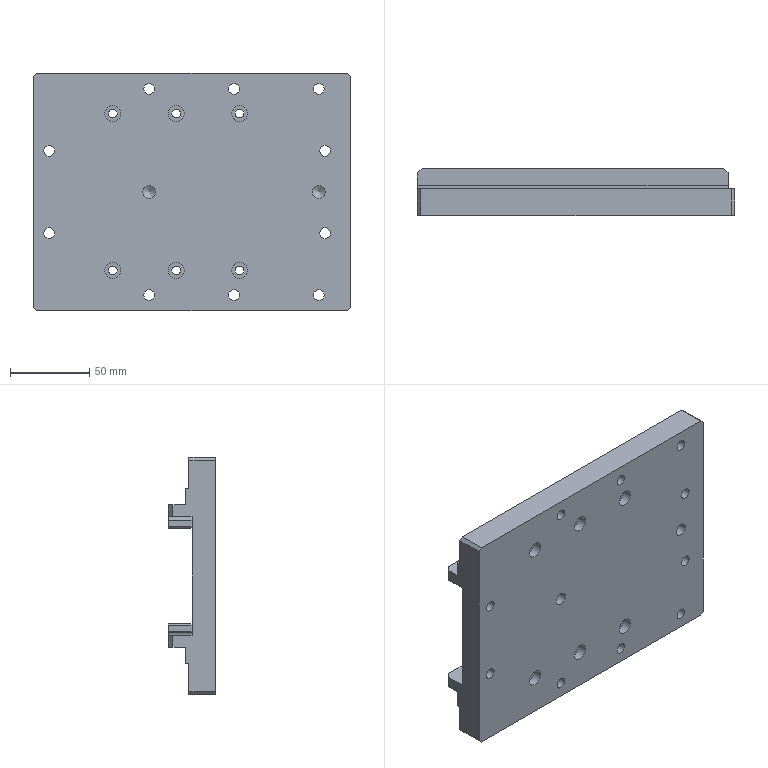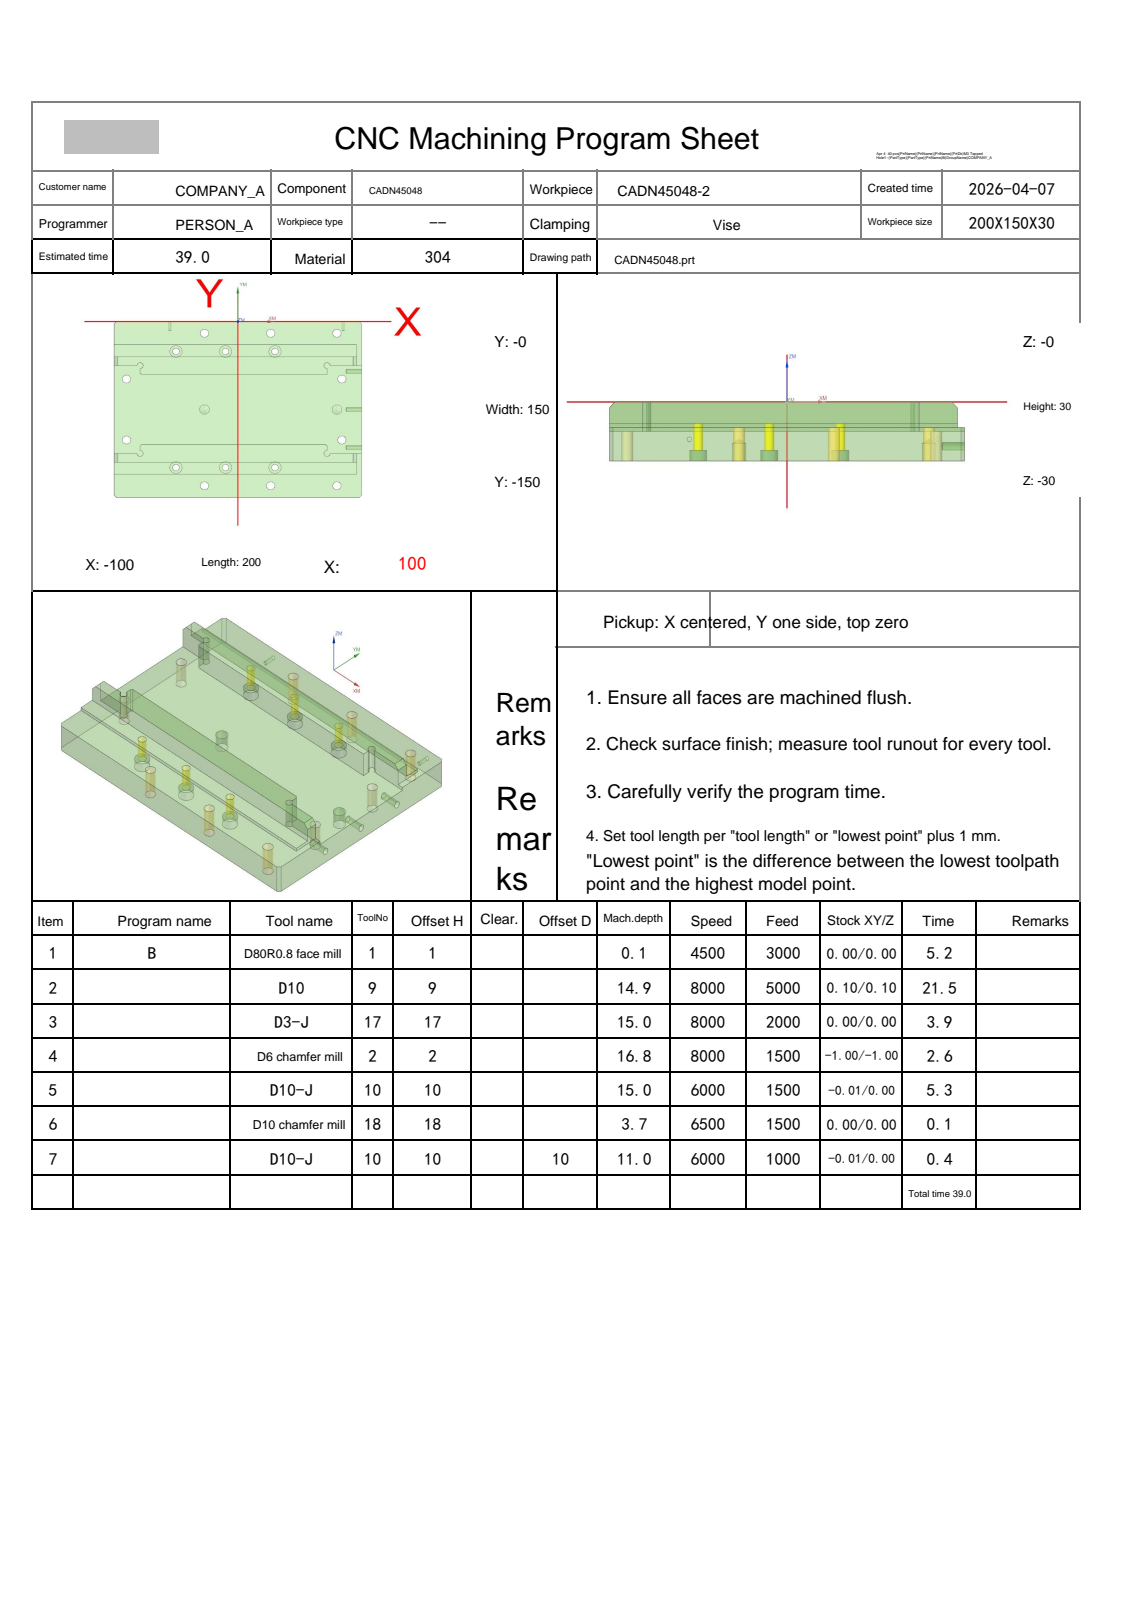NC program | NX | posted by the shop | part box 200 x 30 x 150 mm
Lines 6574 to 7628 of 19220:
N3 T17 M06
(D3-J  D=3. R=0. H=17 ce=0.00 di=0.00)
G00 G90 G54 X77.275 Y-39.301 M03 S8000
G43 H17 Z20.
M08
Z.15
G01 X77.274 Y-39.297 Z.104 F2000.
X77.272 Y-39.286 Z.063
X77.267 Y-39.27 Z.027
X77.26 Y-39.248 Z-.006
X77.251 Y-39.223 Z-.034
X77.239 Y-39.195 Z-.059
X77.224 Y-39.166 Z-.081
X77.206 Y-39.135 Z-.099
X77.185 Y-39.106 Z-.114
X77.16 Y-39.078 Z-.126
X77.131 Y-39.053 Z-.135
X77.099 Y-39.031 Z-.142
X77.062 Y-39.015 Z-.147
X77.021 Y-39.004 Z-.149
X76.975 Y-39. Z-.15
X74.5
G02 X73. Y-37.5 I0.0 J1.5
G03 X72. Y-36.5 I-1. J0.0
X71. Y-37.5 I0.0 J-1.
X72. Y-38.5 I1. J0.0
G02 X73.5 Y-40. I0.0 J-1.5
G01 Y-42.475
X73.514 Y-42.504
X73.555 Y-42.508 Z-.152
X73.619 Y-42.491 Z-.154
X73.705 Y-42.453 Z-.157
X73.809 Y-42.398 Z-.16
X73.929 Y-42.326 Z-.164
X74.202 Y-42.141 Z-.174
X74.38 Y-42.011 Z-.18
X74.671 Y-41.786 Z-.191
X75.106 Y-41.414 Z-.208
X75.528 Y-41.013 Z-.225
X75.93 Y-40.592 Z-.242
X76.299 Y-40.16 Z-.259
X76.522 Y-39.872 Z-.27
X76.65 Y-39.695 Z-.276
X76.832 Y-39.424 Z-.286
X76.902 Y-39.306 Z-.29
X76.957 Y-39.203 Z-.293
X76.993 Y-39.118 Z-.296
X77.009 Y-39.054 Z-.298
X77.004 Y-39.014 Z-.3
X76.975 Y-39.
X74.5
G02 X73. Y-37.5 I0.0 J1.5
G03 X72. Y-36.5 I-1. J0.0
X71. Y-37.5 I0.0 J-1.
X72. Y-38.5 I1. J0.0
G02 X73.5 Y-40. I0.0 J-1.5
G01 Y-42.475
X73.514 Y-42.504
X73.555 Y-42.508 Z-.302
X73.619 Y-42.491 Z-.304
X73.705 Y-42.453 Z-.307
X73.809 Y-42.398 Z-.31
X73.929 Y-42.326 Z-.314
X74.202 Y-42.141 Z-.324
X74.38 Y-42.011 Z-.33
X74.671 Y-41.786 Z-.341
X75.106 Y-41.414 Z-.358
X75.528 Y-41.013 Z-.375
X75.93 Y-40.592 Z-.392
X76.299 Y-40.16 Z-.409
X76.522 Y-39.872 Z-.42
X76.65 Y-39.695 Z-.426
X76.832 Y-39.424 Z-.436
X76.902 Y-39.306 Z-.44
X76.957 Y-39.203 Z-.443
X76.993 Y-39.118 Z-.446
X77.009 Y-39.054 Z-.448
X77.004 Y-39.014 Z-.45
X76.975 Y-39.
X74.5
G02 X73. Y-37.5 I0.0 J1.5
G03 X72. Y-36.5 I-1. J0.0
X71. Y-37.5 I0.0 J-1.
X72. Y-38.5 I1. J0.0
G02 X73.5 Y-40. I0.0 J-1.5
G01 Y-42.475
X73.514 Y-42.504
X73.555 Y-42.508 Z-.452
X73.619 Y-42.491 Z-.454
X73.705 Y-42.453 Z-.457
X73.809 Y-42.398 Z-.46
X73.929 Y-42.326 Z-.464
X74.202 Y-42.141 Z-.474
X74.38 Y-42.011 Z-.48
X74.671 Y-41.786 Z-.491
X75.106 Y-41.414 Z-.508
X75.528 Y-41.013 Z-.525
X75.93 Y-40.592 Z-.542
X76.299 Y-40.16 Z-.559
X76.522 Y-39.872 Z-.57
X76.65 Y-39.695 Z-.576
X76.832 Y-39.424 Z-.586
X76.902 Y-39.306 Z-.59
X76.957 Y-39.203 Z-.593
X76.993 Y-39.118 Z-.596
X77.009 Y-39.054 Z-.598
X77.004 Y-39.014 Z-.6
X76.975 Y-39.
X74.5
G02 X73. Y-37.5 I0.0 J1.5
G03 X72. Y-36.5 I-1. J0.0
X71. Y-37.5 I0.0 J-1.
X72. Y-38.5 I1. J0.0
G02 X73.5 Y-40. I0.0 J-1.5
G01 Y-42.475
X73.514 Y-42.504
X73.555 Y-42.508 Z-.602
X73.619 Y-42.491 Z-.604
X73.705 Y-42.453 Z-.607
X73.809 Y-42.398 Z-.61
X73.929 Y-42.326 Z-.614
X74.202 Y-42.141 Z-.624
X74.38 Y-42.011 Z-.63
X74.671 Y-41.786 Z-.641
X75.106 Y-41.414 Z-.658
X75.528 Y-41.013 Z-.675
X75.93 Y-40.592 Z-.692
X76.299 Y-40.16 Z-.709
X76.522 Y-39.872 Z-.72
X76.65 Y-39.695 Z-.726
X76.832 Y-39.424 Z-.736
X76.902 Y-39.306 Z-.74
X76.957 Y-39.203 Z-.743
X76.993 Y-39.118 Z-.746
X77.009 Y-39.054 Z-.748
X77.004 Y-39.014 Z-.75
X76.975 Y-39.
X74.5
G02 X73. Y-37.5 I0.0 J1.5
G03 X72. Y-36.5 I-1. J0.0
X71. Y-37.5 I0.0 J-1.
X72. Y-38.5 I1. J0.0
G02 X73.5 Y-40. I0.0 J-1.5
G01 Y-42.475
X73.514 Y-42.504
X73.555 Y-42.508 Z-.752
X73.619 Y-42.491 Z-.754
X73.705 Y-42.453 Z-.757
X73.809 Y-42.398 Z-.76
X73.929 Y-42.326 Z-.764
X74.202 Y-42.141 Z-.774
X74.38 Y-42.011 Z-.78
X74.671 Y-41.786 Z-.791
X75.106 Y-41.414 Z-.808
X75.528 Y-41.013 Z-.825
X75.93 Y-40.592 Z-.842
X76.299 Y-40.16 Z-.859
X76.522 Y-39.872 Z-.87
X76.65 Y-39.695 Z-.876
X76.832 Y-39.424 Z-.886
X76.902 Y-39.306 Z-.89
X76.957 Y-39.203 Z-.893
X76.993 Y-39.118 Z-.896
X77.009 Y-39.054 Z-.898
X77.004 Y-39.014 Z-.9
X76.975 Y-39.
X74.5
G02 X73. Y-37.5 I0.0 J1.5
G03 X72. Y-36.5 I-1. J0.0
X71. Y-37.5 I0.0 J-1.
X72. Y-38.5 I1. J0.0
G02 X73.5 Y-40. I0.0 J-1.5
G01 Y-42.475
X73.514 Y-42.504
X73.555 Y-42.508 Z-.902
X73.619 Y-42.491 Z-.904
X73.705 Y-42.453 Z-.907
X73.809 Y-42.398 Z-.91
X73.929 Y-42.326 Z-.914
X74.202 Y-42.141 Z-.924
X74.38 Y-42.011 Z-.93
X74.671 Y-41.786 Z-.941
X75.106 Y-41.414 Z-.958
X75.528 Y-41.013 Z-.975
X75.93 Y-40.592 Z-.992
X76.299 Y-40.16 Z-1.009
X76.522 Y-39.872 Z-1.02
X76.65 Y-39.695 Z-1.026
X76.832 Y-39.424 Z-1.036
X76.902 Y-39.306 Z-1.04
X76.957 Y-39.203 Z-1.043
X76.993 Y-39.118 Z-1.046
X77.009 Y-39.054 Z-1.048
X77.004 Y-39.014 Z-1.05
X76.975 Y-39.
X74.5
G02 X73. Y-37.5 I0.0 J1.5
G03 X72. Y-36.5 I-1. J0.0
X71. Y-37.5 I0.0 J-1.
X72. Y-38.5 I1. J0.0
G02 X73.5 Y-40. I0.0 J-1.5
G01 Y-42.475
X73.514 Y-42.504
X73.555 Y-42.508 Z-1.052
X73.619 Y-42.491 Z-1.054
X73.705 Y-42.453 Z-1.057
X73.809 Y-42.398 Z-1.06
X73.929 Y-42.326 Z-1.064
X74.202 Y-42.141 Z-1.074
X74.38 Y-42.011 Z-1.08
X74.671 Y-41.786 Z-1.091
X75.106 Y-41.414 Z-1.108
X75.528 Y-41.013 Z-1.125
X75.93 Y-40.592 Z-1.142
X76.299 Y-40.16 Z-1.159
X76.522 Y-39.872 Z-1.17
X76.65 Y-39.695 Z-1.176
X76.832 Y-39.424 Z-1.186
X76.902 Y-39.306 Z-1.19
X76.957 Y-39.203 Z-1.193
X76.993 Y-39.118 Z-1.196
X77.009 Y-39.054 Z-1.198
X77.004 Y-39.014 Z-1.2
X76.975 Y-39.
X74.5
G02 X73. Y-37.5 I0.0 J1.5
G03 X72. Y-36.5 I-1. J0.0
X71. Y-37.5 I0.0 J-1.
X72. Y-38.5 I1. J0.0
G02 X73.5 Y-40. I0.0 J-1.5
G01 Y-42.475
X73.514 Y-42.504
X73.555 Y-42.508 Z-1.202
X73.619 Y-42.491 Z-1.204
X73.705 Y-42.453 Z-1.207
X73.809 Y-42.398 Z-1.21
X73.929 Y-42.326 Z-1.214
X74.202 Y-42.141 Z-1.224
X74.38 Y-42.011 Z-1.23
X74.671 Y-41.786 Z-1.241
X75.106 Y-41.414 Z-1.258
X75.528 Y-41.013 Z-1.275
X75.93 Y-40.592 Z-1.292
X76.299 Y-40.16 Z-1.309
X76.522 Y-39.872 Z-1.32
X76.65 Y-39.695 Z-1.326
X76.832 Y-39.424 Z-1.336
X76.902 Y-39.306 Z-1.34
X76.957 Y-39.203 Z-1.343
X76.993 Y-39.118 Z-1.346
X77.009 Y-39.054 Z-1.348
X77.004 Y-39.014 Z-1.35
X76.975 Y-39.
X74.5
G02 X73. Y-37.5 I0.0 J1.5
G03 X72. Y-36.5 I-1. J0.0
X71. Y-37.5 I0.0 J-1.
X72. Y-38.5 I1. J0.0
G02 X73.5 Y-40. I0.0 J-1.5
G01 Y-42.475
X73.514 Y-42.504
X73.555 Y-42.508 Z-1.352
X73.619 Y-42.491 Z-1.354
X73.705 Y-42.453 Z-1.357
X73.809 Y-42.398 Z-1.36
X73.929 Y-42.326 Z-1.364
X74.202 Y-42.141 Z-1.374
X74.38 Y-42.011 Z-1.38
X74.671 Y-41.786 Z-1.391
X75.106 Y-41.414 Z-1.408
X75.528 Y-41.013 Z-1.425
X75.93 Y-40.592 Z-1.442
X76.299 Y-40.16 Z-1.459
X76.522 Y-39.872 Z-1.47
X76.65 Y-39.695 Z-1.476
X76.832 Y-39.424 Z-1.486
X76.902 Y-39.306 Z-1.49
X76.957 Y-39.203 Z-1.493
X76.993 Y-39.118 Z-1.496
X77.009 Y-39.054 Z-1.498
X77.004 Y-39.014 Z-1.5
X76.975 Y-39.
X74.5
G02 X73. Y-37.5 I0.0 J1.5
G03 X72. Y-36.5 I-1. J0.0
X71. Y-37.5 I0.0 J-1.
X72. Y-38.5 I1. J0.0
G02 X73.5 Y-40. I0.0 J-1.5
G01 Y-42.475
X73.514 Y-42.504
X73.555 Y-42.508 Z-1.502
X73.619 Y-42.491 Z-1.504
X73.705 Y-42.453 Z-1.507
X73.809 Y-42.398 Z-1.51
X73.929 Y-42.326 Z-1.514
X74.202 Y-42.141 Z-1.524
X74.38 Y-42.011 Z-1.53
X74.671 Y-41.786 Z-1.541
X75.106 Y-41.414 Z-1.558
X75.528 Y-41.013 Z-1.575
X75.93 Y-40.592 Z-1.592
X76.299 Y-40.16 Z-1.609
X76.522 Y-39.872 Z-1.62
X76.65 Y-39.695 Z-1.626
X76.832 Y-39.424 Z-1.636
X76.902 Y-39.306 Z-1.64
X76.957 Y-39.203 Z-1.643
X76.993 Y-39.118 Z-1.646
X77.009 Y-39.054 Z-1.648
X77.004 Y-39.014 Z-1.65
X76.975 Y-39.
X74.5
G02 X73. Y-37.5 I0.0 J1.5
G03 X72. Y-36.5 I-1. J0.0
X71. Y-37.5 I0.0 J-1.
X72. Y-38.5 I1. J0.0
G02 X73.5 Y-40. I0.0 J-1.5
G01 Y-42.475
X73.514 Y-42.504
X73.555 Y-42.508 Z-1.652
X73.619 Y-42.491 Z-1.654
X73.705 Y-42.453 Z-1.657
X73.809 Y-42.398 Z-1.66
X73.929 Y-42.326 Z-1.664
X74.202 Y-42.141 Z-1.674
X74.38 Y-42.011 Z-1.68
X74.671 Y-41.786 Z-1.691
X75.106 Y-41.414 Z-1.708
X75.528 Y-41.013 Z-1.725
X75.93 Y-40.592 Z-1.742
X76.299 Y-40.16 Z-1.759
X76.522 Y-39.872 Z-1.77
X76.65 Y-39.695 Z-1.776
X76.832 Y-39.424 Z-1.786
X76.902 Y-39.306 Z-1.79
X76.957 Y-39.203 Z-1.793
X76.993 Y-39.118 Z-1.796
X77.009 Y-39.054 Z-1.798
X77.004 Y-39.014 Z-1.8
X76.975 Y-39.
X74.5
G02 X73. Y-37.5 I0.0 J1.5
G03 X72. Y-36.5 I-1. J0.0
X71. Y-37.5 I0.0 J-1.
X72. Y-38.5 I1. J0.0
G02 X73.5 Y-40. I0.0 J-1.5
G01 Y-42.475
X73.514 Y-42.504
X73.555 Y-42.508 Z-1.802
X73.619 Y-42.491 Z-1.804
X73.705 Y-42.453 Z-1.807
X73.809 Y-42.398 Z-1.81
X73.929 Y-42.326 Z-1.814
X74.202 Y-42.141 Z-1.824
X74.38 Y-42.011 Z-1.83
X74.671 Y-41.786 Z-1.841
X75.106 Y-41.414 Z-1.858
X75.528 Y-41.013 Z-1.875
X75.93 Y-40.592 Z-1.892
X76.299 Y-40.16 Z-1.909
X76.522 Y-39.872 Z-1.92
X76.65 Y-39.695 Z-1.926
X76.832 Y-39.424 Z-1.936
X76.902 Y-39.306 Z-1.94
X76.957 Y-39.203 Z-1.943
X76.993 Y-39.118 Z-1.946
X77.009 Y-39.054 Z-1.948
X77.004 Y-39.014 Z-1.95
X76.975 Y-39.
X74.5
G02 X73. Y-37.5 I0.0 J1.5
G03 X72. Y-36.5 I-1. J0.0
X71. Y-37.5 I0.0 J-1.
X72. Y-38.5 I1. J0.0
G02 X73.5 Y-40. I0.0 J-1.5
G01 Y-42.475
X73.514 Y-42.504
X73.555 Y-42.508 Z-1.952
X73.619 Y-42.491 Z-1.954
X73.705 Y-42.453 Z-1.957
X73.809 Y-42.398 Z-1.96
X73.929 Y-42.326 Z-1.964
X74.202 Y-42.141 Z-1.974
X74.38 Y-42.011 Z-1.98
X74.671 Y-41.786 Z-1.991
X75.106 Y-41.414 Z-2.008
X75.528 Y-41.013 Z-2.025
X75.93 Y-40.592 Z-2.042
X76.299 Y-40.16 Z-2.059
X76.522 Y-39.872 Z-2.07
X76.65 Y-39.695 Z-2.076
X76.832 Y-39.424 Z-2.086
X76.902 Y-39.306 Z-2.09
X76.957 Y-39.203 Z-2.093
X76.993 Y-39.118 Z-2.096
X77.009 Y-39.054 Z-2.098
X77.004 Y-39.014 Z-2.1
X76.975 Y-39.
X74.5
G02 X73. Y-37.5 I0.0 J1.5
G03 X72. Y-36.5 I-1. J0.0
X71. Y-37.5 I0.0 J-1.
X72. Y-38.5 I1. J0.0
G02 X73.5 Y-40. I0.0 J-1.5
G01 Y-42.475
X73.514 Y-42.504
X73.555 Y-42.508 Z-2.102
X73.619 Y-42.491 Z-2.104
X73.705 Y-42.453 Z-2.107
X73.809 Y-42.398 Z-2.11
X73.929 Y-42.326 Z-2.114
X74.202 Y-42.141 Z-2.124
X74.38 Y-42.011 Z-2.13
X74.671 Y-41.786 Z-2.141
X75.106 Y-41.414 Z-2.158
X75.528 Y-41.013 Z-2.175
X75.93 Y-40.592 Z-2.192
X76.299 Y-40.16 Z-2.209
X76.522 Y-39.872 Z-2.22
X76.65 Y-39.695 Z-2.226
X76.832 Y-39.424 Z-2.236
X76.902 Y-39.306 Z-2.24
X76.957 Y-39.203 Z-2.243
X76.993 Y-39.118 Z-2.246
X77.009 Y-39.054 Z-2.248
X77.004 Y-39.014 Z-2.25
X76.975 Y-39.
X74.5
G02 X73. Y-37.5 I0.0 J1.5
G03 X72. Y-36.5 I-1. J0.0
X71. Y-37.5 I0.0 J-1.
X72. Y-38.5 I1. J0.0
G02 X73.5 Y-40. I0.0 J-1.5
G01 Y-42.475
X73.514 Y-42.504
X73.555 Y-42.508 Z-2.252
X73.619 Y-42.491 Z-2.254
X73.705 Y-42.453 Z-2.257
X73.809 Y-42.398 Z-2.26
X73.929 Y-42.326 Z-2.264
X74.202 Y-42.141 Z-2.274
X74.38 Y-42.011 Z-2.28
X74.671 Y-41.786 Z-2.291
X75.106 Y-41.414 Z-2.308
X75.528 Y-41.013 Z-2.325
X75.93 Y-40.592 Z-2.342
X76.299 Y-40.16 Z-2.359
X76.522 Y-39.872 Z-2.37
X76.65 Y-39.695 Z-2.376
X76.832 Y-39.424 Z-2.386
X76.902 Y-39.306 Z-2.39
X76.957 Y-39.203 Z-2.393
X76.993 Y-39.118 Z-2.396
X77.009 Y-39.054 Z-2.398
X77.004 Y-39.014 Z-2.4
X76.975 Y-39.
X74.5
G02 X73. Y-37.5 I0.0 J1.5
G03 X72. Y-36.5 I-1. J0.0
X71. Y-37.5 I0.0 J-1.
X72. Y-38.5 I1. J0.0
G02 X73.5 Y-40. I0.0 J-1.5
G01 Y-42.475
X73.514 Y-42.504
X73.555 Y-42.508 Z-2.402
X73.619 Y-42.491 Z-2.404
X73.705 Y-42.453 Z-2.407
X73.809 Y-42.398 Z-2.41
X73.929 Y-42.326 Z-2.414
X74.202 Y-42.141 Z-2.424
X74.38 Y-42.011 Z-2.43
X74.671 Y-41.786 Z-2.441
X75.106 Y-41.414 Z-2.458
X75.528 Y-41.013 Z-2.475
X75.93 Y-40.592 Z-2.492
X76.299 Y-40.16 Z-2.509
X76.522 Y-39.872 Z-2.52
X76.65 Y-39.695 Z-2.526
X76.832 Y-39.424 Z-2.536
X76.902 Y-39.306 Z-2.54
X76.957 Y-39.203 Z-2.543
X76.993 Y-39.118 Z-2.546
X77.009 Y-39.054 Z-2.548
X77.004 Y-39.014 Z-2.55
X76.975 Y-39.
X74.5
G02 X73. Y-37.5 I0.0 J1.5
G03 X72. Y-36.5 I-1. J0.0
X71. Y-37.5 I0.0 J-1.
X72. Y-38.5 I1. J0.0
G02 X73.5 Y-40. I0.0 J-1.5
G01 Y-42.475
X73.514 Y-42.504
X73.555 Y-42.508 Z-2.552
X73.619 Y-42.491 Z-2.554
X73.705 Y-42.453 Z-2.557
X73.809 Y-42.398 Z-2.56
X73.929 Y-42.326 Z-2.564
X74.202 Y-42.141 Z-2.574
X74.38 Y-42.011 Z-2.58
X74.671 Y-41.786 Z-2.591
X75.106 Y-41.414 Z-2.608
X75.528 Y-41.013 Z-2.625
X75.93 Y-40.592 Z-2.642
X76.299 Y-40.16 Z-2.659
X76.522 Y-39.872 Z-2.67
X76.65 Y-39.695 Z-2.676
X76.832 Y-39.424 Z-2.686
X76.902 Y-39.306 Z-2.69
X76.957 Y-39.203 Z-2.693
X76.993 Y-39.118 Z-2.696
X77.009 Y-39.054 Z-2.698
X77.004 Y-39.014 Z-2.7
X76.975 Y-39.
X74.5
G02 X73. Y-37.5 I0.0 J1.5
G03 X72. Y-36.5 I-1. J0.0
X71. Y-37.5 I0.0 J-1.
X72. Y-38.5 I1. J0.0
G02 X73.5 Y-40. I0.0 J-1.5
G01 Y-42.475
X73.514 Y-42.504
X73.555 Y-42.508 Z-2.702
X73.619 Y-42.491 Z-2.704
X73.705 Y-42.453 Z-2.707
X73.809 Y-42.398 Z-2.71
X73.929 Y-42.326 Z-2.714
X74.202 Y-42.141 Z-2.724
X74.38 Y-42.011 Z-2.73
X74.671 Y-41.786 Z-2.741
X75.106 Y-41.414 Z-2.758
X75.528 Y-41.013 Z-2.775
X75.93 Y-40.592 Z-2.792
X76.299 Y-40.16 Z-2.809
X76.522 Y-39.872 Z-2.82
X76.65 Y-39.695 Z-2.826
X76.832 Y-39.424 Z-2.836
X76.902 Y-39.306 Z-2.84
X76.957 Y-39.203 Z-2.843
X76.993 Y-39.118 Z-2.846
X77.009 Y-39.054 Z-2.848
X77.004 Y-39.014 Z-2.85
X76.975 Y-39.
X74.5
G02 X73. Y-37.5 I0.0 J1.5
G03 X72. Y-36.5 I-1. J0.0
X71. Y-37.5 I0.0 J-1.
X72. Y-38.5 I1. J0.0
G02 X73.5 Y-40. I0.0 J-1.5
G01 Y-42.475
X73.514 Y-42.504
X73.555 Y-42.508 Z-2.852
X73.619 Y-42.491 Z-2.854
X73.705 Y-42.453 Z-2.857
X73.809 Y-42.398 Z-2.86
X73.929 Y-42.326 Z-2.864
X74.202 Y-42.141 Z-2.874
X74.38 Y-42.011 Z-2.88
X74.671 Y-41.786 Z-2.891
X75.106 Y-41.414 Z-2.908
X75.528 Y-41.013 Z-2.925
X75.93 Y-40.592 Z-2.942
X76.299 Y-40.16 Z-2.959
X76.522 Y-39.872 Z-2.97
X76.65 Y-39.695 Z-2.976
X76.832 Y-39.424 Z-2.986
X76.902 Y-39.306 Z-2.99
X76.957 Y-39.203 Z-2.993
X76.993 Y-39.118 Z-2.996
X77.009 Y-39.054 Z-2.998
X77.004 Y-39.014 Z-3.
X76.975 Y-39.
X74.5
G02 X73. Y-37.5 I0.0 J1.5
G03 X72. Y-36.5 I-1. J0.0
X71. Y-37.5 I0.0 J-1.
X72. Y-38.5 I1. J0.0
G02 X73.5 Y-40. I0.0 J-1.5
G01 Y-42.475
X73.514 Y-42.504
X73.555 Y-42.508 Z-3.002
X73.619 Y-42.491 Z-3.004
X73.705 Y-42.453 Z-3.007
X73.809 Y-42.398 Z-3.01
X73.929 Y-42.326 Z-3.014
X74.202 Y-42.141 Z-3.024
X74.38 Y-42.011 Z-3.03
X74.671 Y-41.786 Z-3.041
X75.106 Y-41.415 Z-3.058
X75.528 Y-41.014 Z-3.075
X75.93 Y-40.593 Z-3.092
X76.299 Y-40.161 Z-3.109
X76.522 Y-39.872 Z-3.12
X76.65 Y-39.695 Z-3.126
X76.832 Y-39.425 Z-3.136
X76.902 Y-39.306 Z-3.14
X76.957 Y-39.203 Z-3.143
X76.993 Y-39.118 Z-3.146
X77.009 Y-39.054 Z-3.148
X77.004 Y-39.014 Z-3.15
X76.975 Y-39.
X74.5
G02 X73. Y-37.5 I0.0 J1.5
G03 X72. Y-36.5 I-1. J0.0
X71. Y-37.5 I0.0 J-1.
X72. Y-38.5 I1. J0.0
G02 X73.5 Y-40. I0.0 J-1.5
G01 Y-42.475
X73.514 Y-42.504
X73.555 Y-42.508 Z-3.152
X73.619 Y-42.491 Z-3.154
X73.705 Y-42.453 Z-3.157
X73.809 Y-42.398 Z-3.16
X73.929 Y-42.326 Z-3.164
X74.202 Y-42.141 Z-3.174
X74.38 Y-42.011 Z-3.18
X74.671 Y-41.786 Z-3.191
X75.106 Y-41.415 Z-3.208
X75.528 Y-41.014 Z-3.225
X75.93 Y-40.593 Z-3.242
X76.299 Y-40.161 Z-3.259
X76.522 Y-39.872 Z-3.27
X76.65 Y-39.695 Z-3.276
X76.832 Y-39.425 Z-3.286
X76.902 Y-39.306 Z-3.29
X76.957 Y-39.203 Z-3.293
X76.993 Y-39.118 Z-3.296
X77.009 Y-39.054 Z-3.298
X77.004 Y-39.014 Z-3.3
X76.975 Y-39.
X74.5
G02 X73. Y-37.5 I0.0 J1.5
G03 X72. Y-36.5 I-1. J0.0
X71. Y-37.5 I0.0 J-1.
X72. Y-38.5 I1. J0.0
G02 X73.5 Y-40. I0.0 J-1.5
G01 Y-42.475
X73.514 Y-42.504
X73.555 Y-42.508 Z-3.302
X73.619 Y-42.491 Z-3.304
X73.705 Y-42.453 Z-3.307
X73.809 Y-42.398 Z-3.31
X73.929 Y-42.326 Z-3.314
X74.202 Y-42.141 Z-3.324
X74.38 Y-42.011 Z-3.33
X74.671 Y-41.786 Z-3.341
X75.106 Y-41.415 Z-3.358
X75.528 Y-41.014 Z-3.375
X75.93 Y-40.593 Z-3.392
X76.299 Y-40.161 Z-3.409
X76.522 Y-39.872 Z-3.42
X76.65 Y-39.695 Z-3.426
X76.832 Y-39.425 Z-3.436
X76.902 Y-39.306 Z-3.44
X76.957 Y-39.203 Z-3.443
X76.993 Y-39.118 Z-3.446
X77.009 Y-39.054 Z-3.448
X77.004 Y-39.014 Z-3.45
X76.975 Y-39.
X74.5
G02 X73. Y-37.5 I0.0 J1.5
G03 X72. Y-36.5 I-1. J0.0
X71. Y-37.5 I0.0 J-1.
X72. Y-38.5 I1. J0.0
G02 X73.5 Y-40. I0.0 J-1.5
G01 Y-42.475
X73.514 Y-42.504
X73.555 Y-42.508 Z-3.452
X73.619 Y-42.491 Z-3.454
X73.705 Y-42.453 Z-3.457
X73.809 Y-42.398 Z-3.46
X73.929 Y-42.326 Z-3.464
X74.202 Y-42.141 Z-3.474
X74.38 Y-42.011 Z-3.48
X74.671 Y-41.786 Z-3.491
X75.106 Y-41.415 Z-3.508
X75.528 Y-41.014 Z-3.525
X75.93 Y-40.593 Z-3.542
X76.299 Y-40.161 Z-3.559
X76.522 Y-39.872 Z-3.57
X76.65 Y-39.695 Z-3.576
X76.832 Y-39.425 Z-3.586
X76.902 Y-39.306 Z-3.59
X76.957 Y-39.203 Z-3.593
X76.993 Y-39.118 Z-3.596
X77.009 Y-39.054 Z-3.598
X77.004 Y-39.014 Z-3.6
X76.975 Y-39.
X74.5
G02 X73. Y-37.5 I0.0 J1.5
G03 X72. Y-36.5 I-1. J0.0
X71. Y-37.5 I0.0 J-1.
X72. Y-38.5 I1. J0.0
G02 X73.5 Y-40. I0.0 J-1.5
G01 Y-42.475
X73.514 Y-42.504
X73.555 Y-42.508 Z-3.602
X73.619 Y-42.491 Z-3.604
X73.705 Y-42.453 Z-3.607
X73.809 Y-42.398 Z-3.61
X73.929 Y-42.326 Z-3.614
X74.202 Y-42.141 Z-3.624
X74.38 Y-42.011 Z-3.63
X74.671 Y-41.786 Z-3.641
X75.106 Y-41.415 Z-3.658
X75.528 Y-41.014 Z-3.675
X75.93 Y-40.593 Z-3.692
X76.299 Y-40.161 Z-3.709
X76.522 Y-39.872 Z-3.72
X76.65 Y-39.695 Z-3.726
X76.832 Y-39.425 Z-3.736
X76.902 Y-39.306 Z-3.74
X76.957 Y-39.203 Z-3.743
X76.993 Y-39.118 Z-3.746
X77.009 Y-39.054 Z-3.748
X77.004 Y-39.014 Z-3.75
X76.975 Y-39.
X74.5
G02 X73. Y-37.5 I0.0 J1.5
G03 X72. Y-36.5 I-1. J0.0
X71. Y-37.5 I0.0 J-1.
X72. Y-38.5 I1. J0.0
G02 X73.5 Y-40. I0.0 J-1.5
G01 Y-42.475
X73.514 Y-42.504
X73.555 Y-42.508 Z-3.752
X73.619 Y-42.491 Z-3.754
X73.705 Y-42.453 Z-3.757
X73.809 Y-42.398 Z-3.76
X73.929 Y-42.326 Z-3.764
X74.202 Y-42.141 Z-3.774
X74.38 Y-42.011 Z-3.78
X74.671 Y-41.786 Z-3.791
X75.106 Y-41.415 Z-3.808
X75.528 Y-41.014 Z-3.825
X75.93 Y-40.593 Z-3.842
X76.299 Y-40.161 Z-3.859
X76.522 Y-39.872 Z-3.87
X76.65 Y-39.695 Z-3.876
X76.832 Y-39.425 Z-3.886
X76.902 Y-39.306 Z-3.89
X76.957 Y-39.203 Z-3.893
X76.993 Y-39.118 Z-3.896
X77.009 Y-39.054 Z-3.898
X77.004 Y-39.014 Z-3.9
X76.975 Y-39.
X74.5
G02 X73. Y-37.5 I0.0 J1.5
G03 X72. Y-36.5 I-1. J0.0
X71. Y-37.5 I0.0 J-1.
X72. Y-38.5 I1. J0.0
G02 X73.5 Y-40. I0.0 J-1.5
G01 Y-42.475
X73.514 Y-42.504
X73.555 Y-42.508 Z-3.902
X73.619 Y-42.491 Z-3.904
X73.705 Y-42.453 Z-3.907
X73.809 Y-42.398 Z-3.91
X73.929 Y-42.326 Z-3.914
X74.202 Y-42.141 Z-3.924
X74.38 Y-42.011 Z-3.93
X74.671 Y-41.786 Z-3.941
X75.106 Y-41.415 Z-3.958
X75.528 Y-41.014 Z-3.975
X75.93 Y-40.593 Z-3.992
X76.299 Y-40.161 Z-4.009
X76.522 Y-39.872 Z-4.02
X76.65 Y-39.695 Z-4.026
X76.832 Y-39.425 Z-4.036
X76.902 Y-39.306 Z-4.04
X76.957 Y-39.203 Z-4.043
X76.993 Y-39.118 Z-4.046
X77.009 Y-39.054 Z-4.048
X77.004 Y-39.014 Z-4.05
X76.975 Y-39.
X74.5
G02 X73. Y-37.5 I0.0 J1.5
G03 X72. Y-36.5 I-1. J0.0
X71. Y-37.5 I0.0 J-1.
X72. Y-38.5 I1. J0.0
G02 X73.5 Y-40. I0.0 J-1.5
G01 Y-42.475
X73.514 Y-42.504
X73.555 Y-42.508 Z-4.052
X73.619 Y-42.491 Z-4.054
X73.705 Y-42.453 Z-4.057
X73.809 Y-42.398 Z-4.06
X73.929 Y-42.326 Z-4.064
X74.202 Y-42.141 Z-4.074
X74.38 Y-42.011 Z-4.08
X74.671 Y-41.786 Z-4.091
X75.106 Y-41.415 Z-4.108
X75.528 Y-41.014 Z-4.125
X75.93 Y-40.593 Z-4.142
X76.299 Y-40.161 Z-4.159
X76.522 Y-39.872 Z-4.17
X76.65 Y-39.695 Z-4.176
X76.832 Y-39.425 Z-4.186
X76.902 Y-39.306 Z-4.19
X76.957 Y-39.203 Z-4.193
X76.993 Y-39.118 Z-4.196
X77.009 Y-39.054 Z-4.198
X77.004 Y-39.014 Z-4.2
X76.975 Y-39.
X74.5
G02 X73. Y-37.5 I0.0 J1.5
G03 X72. Y-36.5 I-1. J0.0
X71. Y-37.5 I0.0 J-1.
X72. Y-38.5 I1. J0.0
G02 X73.5 Y-40. I0.0 J-1.5
G01 Y-42.475
X73.514 Y-42.504
X73.555 Y-42.508 Z-4.202
X73.619 Y-42.491 Z-4.204
X73.705 Y-42.453 Z-4.207
X73.809 Y-42.398 Z-4.21
X73.929 Y-42.326 Z-4.214
X74.202 Y-42.141 Z-4.224
X74.38 Y-42.011 Z-4.23
X74.671 Y-41.786 Z-4.241
X75.106 Y-41.415 Z-4.258
X75.528 Y-41.014 Z-4.275
X75.93 Y-40.593 Z-4.292
X76.299 Y-40.161 Z-4.309
X76.522 Y-39.872 Z-4.32
X76.65 Y-39.695 Z-4.326
X76.832 Y-39.425 Z-4.336
X76.902 Y-39.306 Z-4.34
X76.957 Y-39.203 Z-4.343
X76.993 Y-39.118 Z-4.346
X77.009 Y-39.054 Z-4.348
X77.004 Y-39.014 Z-4.35
X76.975 Y-39.
X74.5
G02 X73. Y-37.5 I0.0 J1.5
G03 X72. Y-36.5 I-1. J0.0
X71. Y-37.5 I0.0 J-1.
X72. Y-38.5 I1. J0.0
G02 X73.5 Y-40. I0.0 J-1.5
G01 Y-42.475
X73.514 Y-42.504
X73.555 Y-42.508 Z-4.352
X73.619 Y-42.491 Z-4.354
X73.705 Y-42.453 Z-4.357
X73.809 Y-42.398 Z-4.36
X73.929 Y-42.326 Z-4.364
X74.202 Y-42.141 Z-4.374
X74.38 Y-42.011 Z-4.38
X74.671 Y-41.786 Z-4.391
X75.106 Y-41.415 Z-4.408
X75.528 Y-41.014 Z-4.425
X75.93 Y-40.593 Z-4.442
X76.299 Y-40.161 Z-4.459
X76.522 Y-39.872 Z-4.47
X76.65 Y-39.695 Z-4.476
X76.832 Y-39.425 Z-4.486
X76.902 Y-39.306 Z-4.49
X76.957 Y-39.203 Z-4.493
X76.993 Y-39.118 Z-4.496
X77.009 Y-39.054 Z-4.498
X77.004 Y-39.014 Z-4.5
X76.975 Y-39.
X74.5
G02 X73. Y-37.5 I0.0 J1.5
G03 X72. Y-36.5 I-1. J0.0
X71. Y-37.5 I0.0 J-1.
X72. Y-38.5 I1. J0.0
G02 X73.5 Y-40. I0.0 J-1.5
G01 Y-42.475
X73.514 Y-42.504
X73.555 Y-42.508 Z-4.502
X73.619 Y-42.491 Z-4.504
X73.705 Y-42.453 Z-4.507
X73.809 Y-42.398 Z-4.51
X73.929 Y-42.326 Z-4.514
X74.202 Y-42.141 Z-4.524
X74.38 Y-42.011 Z-4.53
X74.671 Y-41.786 Z-4.541
X75.106 Y-41.415 Z-4.558
X75.528 Y-41.014 Z-4.575
X75.93 Y-40.593 Z-4.592
X76.299 Y-40.161 Z-4.609
X76.522 Y-39.872 Z-4.62
X76.65 Y-39.695 Z-4.626
X76.832 Y-39.425 Z-4.636
X76.902 Y-39.306 Z-4.64
X76.957 Y-39.203 Z-4.643
X76.993 Y-39.118 Z-4.646
X77.009 Y-39.054 Z-4.648
X77.004 Y-39.014 Z-4.65
X76.975 Y-39.
X74.5
G02 X73. Y-37.5 I0.0 J1.5
G03 X72. Y-36.5 I-1. J0.0
X71. Y-37.5 I0.0 J-1.
X72. Y-38.5 I1. J0.0
G02 X73.5 Y-40. I0.0 J-1.5
G01 Y-42.475
X73.514 Y-42.504
X73.555 Y-42.508 Z-4.652
X73.619 Y-42.491 Z-4.654
X73.705 Y-42.453 Z-4.657
X73.809 Y-42.398 Z-4.66
X73.929 Y-42.326 Z-4.664
X74.202 Y-42.141 Z-4.674
X74.38 Y-42.011 Z-4.68
X74.671 Y-41.786 Z-4.691
X75.106 Y-41.415 Z-4.708
X75.528 Y-41.014 Z-4.725
X75.93 Y-40.593 Z-4.742
X76.299 Y-40.161 Z-4.759
X76.522 Y-39.872 Z-4.77
X76.65 Y-39.695 Z-4.776
X76.832 Y-39.425 Z-4.786
X76.902 Y-39.306 Z-4.79
X76.957 Y-39.203 Z-4.793
X76.993 Y-39.118 Z-4.796
X77.009 Y-39.054 Z-4.798
X77.004 Y-39.014 Z-4.8
X76.975 Y-39.
X74.5
G02 X73. Y-37.5 I0.0 J1.5
G03 X72. Y-36.5 I-1. J0.0
X71. Y-37.5 I0.0 J-1.
X72. Y-38.5 I1. J0.0
G02 X73.5 Y-40. I0.0 J-1.5
G01 Y-42.475
X73.514 Y-42.504
X73.555 Y-42.508 Z-4.802
X73.619 Y-42.491 Z-4.804
X73.705 Y-42.453 Z-4.807
X73.809 Y-42.398 Z-4.81
X73.929 Y-42.326 Z-4.814
X74.202 Y-42.141 Z-4.824
X74.38 Y-42.011 Z-4.83
X74.671 Y-41.786 Z-4.841
X75.106 Y-41.415 Z-4.858
X75.528 Y-41.014 Z-4.875
X75.93 Y-40.593 Z-4.892
X76.299 Y-40.161 Z-4.909
X76.522 Y-39.872 Z-4.92
X76.65 Y-39.695 Z-4.926
X76.832 Y-39.425 Z-4.936
X76.902 Y-39.306 Z-4.94
X76.957 Y-39.203 Z-4.943
X76.993 Y-39.118 Z-4.946
X77.009 Y-39.054 Z-4.948
X77.004 Y-39.014 Z-4.95
X76.975 Y-39.
X74.5
G02 X73. Y-37.5 I0.0 J1.5
G03 X72. Y-36.5 I-1. J0.0
X71. Y-37.5 I0.0 J-1.
X72. Y-38.5 I1. J0.0
G02 X73.5 Y-40. I0.0 J-1.5
G01 Y-42.475
X73.514 Y-42.504
X73.555 Y-42.508 Z-4.952
X73.619 Y-42.491 Z-4.954
X73.705 Y-42.453 Z-4.957
X73.809 Y-42.398 Z-4.96
X73.929 Y-42.326 Z-4.964
X74.202 Y-42.141 Z-4.974
X74.38 Y-42.011 Z-4.98
X74.671 Y-41.786 Z-4.991
X75.106 Y-41.415 Z-5.008
X75.528 Y-41.014 Z-5.025
X75.93 Y-40.593 Z-5.042
X76.299 Y-40.161 Z-5.059
X76.522 Y-39.872 Z-5.07
X76.65 Y-39.695 Z-5.076
X76.832 Y-39.425 Z-5.086
X76.902 Y-39.306 Z-5.09
X76.957 Y-39.203 Z-5.093
X76.993 Y-39.118 Z-5.096
X77.009 Y-39.054 Z-5.098
X77.004 Y-39.014 Z-5.1
X76.975 Y-39.
X74.5
G02 X73. Y-37.5 I0.0 J1.5
G03 X72. Y-36.5 I-1. J0.0
X71. Y-37.5 I0.0 J-1.
X72. Y-38.5 I1. J0.0
G02 X73.5 Y-40. I0.0 J-1.5
G01 Y-42.475
X73.514 Y-42.504
X73.555 Y-42.508 Z-5.102
X73.619 Y-42.491 Z-5.104
X73.705 Y-42.453 Z-5.107
X73.809 Y-42.398 Z-5.11
X73.929 Y-42.326 Z-5.114
X74.202 Y-42.141 Z-5.124
X74.38 Y-42.011 Z-5.13
X74.671 Y-41.786 Z-5.141
X75.106 Y-41.415 Z-5.158
X75.528 Y-41.014 Z-5.175
X75.93 Y-40.593 Z-5.192
X76.299 Y-40.161 Z-5.209
X76.522 Y-39.872 Z-5.22
X76.65 Y-39.695 Z-5.226
X76.832 Y-39.425 Z-5.236
X76.902 Y-39.306 Z-5.24
X76.957 Y-39.203 Z-5.243
X76.993 Y-39.118 Z-5.246
X77.009 Y-39.054 Z-5.248
X77.004 Y-39.014 Z-5.25
X76.975 Y-39.
X74.5
G02 X73. Y-37.5 I0.0 J1.5
G03 X72. Y-36.5 I-1. J0.0
X71. Y-37.5 I0.0 J-1.
X72. Y-38.5 I1. J0.0
G02 X73.5 Y-40. I0.0 J-1.5
G01 Y-42.475
X73.514 Y-42.504
X73.555 Y-42.508 Z-5.252
X73.619 Y-42.491 Z-5.254
X73.705 Y-42.453 Z-5.257
X73.809 Y-42.398 Z-5.26
X73.929 Y-42.326 Z-5.264
X74.202 Y-42.141 Z-5.274
X74.38 Y-42.011 Z-5.28
X74.671 Y-41.786 Z-5.291
X75.106 Y-41.415 Z-5.308
X75.528 Y-41.014 Z-5.325
X75.93 Y-40.593 Z-5.342
X76.299 Y-40.161 Z-5.359
X76.522 Y-39.872 Z-5.37
X76.65 Y-39.695 Z-5.376
X76.832 Y-39.425 Z-5.386
X76.902 Y-39.306 Z-5.39
X76.957 Y-39.203 Z-5.393
X76.993 Y-39.118 Z-5.396
X77.009 Y-39.054 Z-5.398
X77.004 Y-39.014 Z-5.4
X76.975 Y-39.
X74.5
G02 X73. Y-37.5 I0.0 J1.5
G03 X72. Y-36.5 I-1. J0.0
X71. Y-37.5 I0.0 J-1.
X72. Y-38.5 I1. J0.0
G02 X73.5 Y-40. I0.0 J-1.5
G01 Y-42.475
X73.514 Y-42.504
X73.555 Y-42.508 Z-5.402
X73.619 Y-42.491 Z-5.404
X73.705 Y-42.453 Z-5.407
X73.809 Y-42.398 Z-5.41
X73.929 Y-42.326 Z-5.414
X74.202 Y-42.141 Z-5.424
X74.38 Y-42.011 Z-5.43
X74.671 Y-41.786 Z-5.441
X75.106 Y-41.415 Z-5.458
X75.528 Y-41.014 Z-5.475
X75.93 Y-40.593 Z-5.492